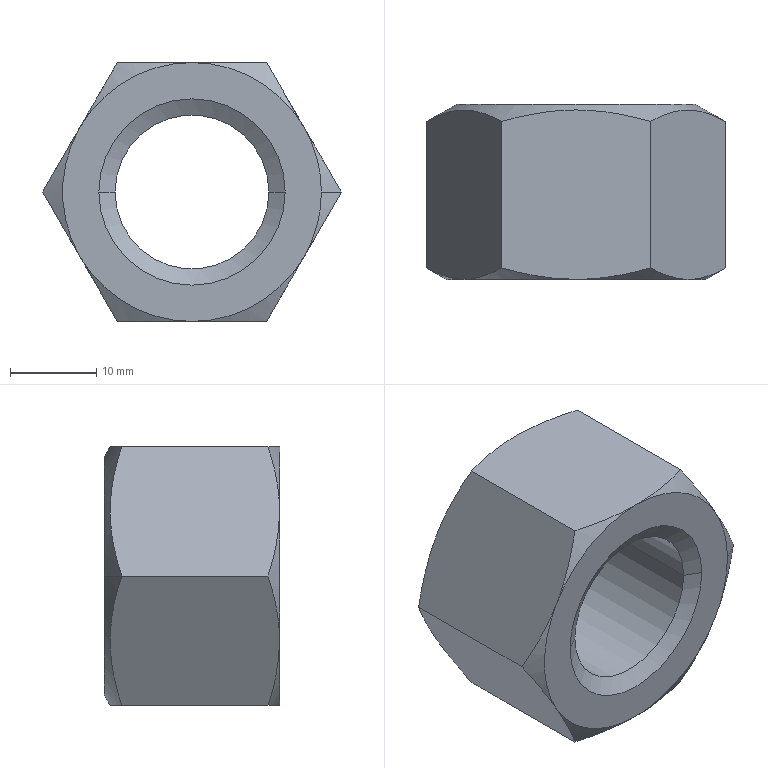Part | NX | features BREP 1 | 1 solid | 23 faces | box 34.641 x 20.3 x 30 mm | volume 10440 mm3 | cone 13 | plane 8 | cylinder 2 | commonest cylinder face diameters 17.835 x2
STEP:
#1=CARTESIAN_POINT('',(58.633,284.435,-38.1));
#2=VERTEX_POINT('',#1);
#3=CARTESIAN_POINT('',(76.468,284.435,-38.1));
#4=VERTEX_POINT('',#3);
#5=CARTESIAN_POINT('',(67.55,284.435,-38.1));
#6=DIRECTION('',(0.,1.,0.));
#7=DIRECTION('',(1.,0.,0.));
#8=AXIS2_PLACEMENT_3D('',#5,#6,#7);
#9=CIRCLE('',#8,8.918);
#10=EDGE_CURVE('',#2,#4,#9,.T.);
#11=ORIENTED_EDGE('',*,*,#10,.F.);
#12=CARTESIAN_POINT('',(56.75,286.317,-38.1));
#13=VERTEX_POINT('',#12);
#14=CARTESIAN_POINT('',(58.633,284.435,-38.1));
#15=DIRECTION('',(-0.7071,0.7071,0.));
#16=VECTOR('',#15,1000.);
#17=LINE('',#14,#16);
#18=EDGE_CURVE('',#2,#13,#17,.T.);
#19=ORIENTED_EDGE('',*,*,#18,.T.);
#20=CARTESIAN_POINT('',(78.35,286.317,-38.1));
#21=VERTEX_POINT('',#20);
#22=CARTESIAN_POINT('',(67.55,286.317,-38.1));
#23=DIRECTION('',(0.,-1.,0.));
#24=DIRECTION('',(1.,0.,0.));
#25=AXIS2_PLACEMENT_3D('',#22,#23,#24);
#26=CIRCLE('',#25,10.8);
#27=EDGE_CURVE('',#21,#13,#26,.T.);
#28=ORIENTED_EDGE('',*,*,#27,.F.);
#29=CARTESIAN_POINT('',(76.468,284.435,-38.1));
#30=DIRECTION('',(0.7071,0.7071,0.));
#31=VECTOR('',#30,1000.);
#32=LINE('',#29,#31);
#33=EDGE_CURVE('',#4,#21,#32,.T.);
#34=ORIENTED_EDGE('',*,*,#33,.F.);
#35=EDGE_LOOP('',(#11,#19,#28,#34));
#36=FACE_BOUND('',#35,.T.);
#37=CARTESIAN_POINT('',(67.55,284.435,-38.1));
#38=DIRECTION('',(0.,1.,0.));
#39=DIRECTION('',(-1.,0.,0.));
#40=AXIS2_PLACEMENT_3D('',#37,#38,#39);
#41=CONICAL_SURFACE('',#40,8.918,0.7854);
#42=ADVANCED_FACE('',(#36),#41,.F.);
#43=CARTESIAN_POINT('',(53.7,286.317,-38.1));
#44=VERTEX_POINT('',#43);
#45=CARTESIAN_POINT('',(81.4,286.317,-38.1));
#46=VERTEX_POINT('',#45);
#47=CARTESIAN_POINT('',(67.55,286.317,-38.1));
#48=DIRECTION('',(0.,-1.,0.));
#49=DIRECTION('',(-1.,0.,0.));
#50=AXIS2_PLACEMENT_3D('',#47,#48,#49);
#51=CIRCLE('',#50,13.85);
#52=EDGE_CURVE('',#44,#46,#51,.T.);
#53=ORIENTED_EDGE('',*,*,#52,.T.);
#54=CARTESIAN_POINT('',(84.871,284.314,-38.1));
#55=VERTEX_POINT('',#54);
#56=CARTESIAN_POINT('',(84.871,284.314,-38.1));
#57=DIRECTION('',(0.866,-0.5,0.));
#58=VECTOR('',#57,1000.);
#59=LINE('',#56,#58);
#60=EDGE_CURVE('',#55,#46,#59,.F.);
#61=ORIENTED_EDGE('',*,*,#60,.F.);
#62=CARTESIAN_POINT('',(76.21,284.314,-53.1));
#63=VERTEX_POINT('',#62);
#64=CARTESIAN_POINT('',(76.21,284.314,-53.1));
#65=CARTESIAN_POINT('',(77.624,285.13,-50.651));
#66=CARTESIAN_POINT('',(80.525,286.176,-45.627));
#67=CARTESIAN_POINT('',(83.455,285.131,-40.552));
#68=CARTESIAN_POINT('',(84.871,284.314,-38.1));
#69=B_SPLINE_CURVE_WITH_KNOTS('',3,(#64,#65,#66,#67,#68),.UNSPECIFIED.,.F.,.F.,(4,1,4),(0.,0.008746,0.01749),.UNSPECIFIED.);
#70=EDGE_CURVE('',#63,#55,#69,.T.);
#71=ORIENTED_EDGE('',*,*,#70,.F.);
#72=CARTESIAN_POINT('',(58.89,284.314,-53.1));
#73=VERTEX_POINT('',#72);
#74=CARTESIAN_POINT('',(58.89,284.314,-53.1));
#75=CARTESIAN_POINT('',(61.718,285.13,-53.1));
#76=CARTESIAN_POINT('',(67.519,286.176,-53.1));
#77=CARTESIAN_POINT('',(73.379,285.131,-53.1));
#78=CARTESIAN_POINT('',(76.21,284.314,-53.1));
#79=B_SPLINE_CURVE_WITH_KNOTS('',3,(#74,#75,#76,#77,#78),.UNSPECIFIED.,.F.,.F.,(4,1,4),(0.,0.008746,0.01749),.UNSPECIFIED.);
#80=EDGE_CURVE('',#73,#63,#79,.T.);
#81=ORIENTED_EDGE('',*,*,#80,.F.);
#82=CARTESIAN_POINT('',(50.229,284.314,-38.1));
#83=VERTEX_POINT('',#82);
#84=CARTESIAN_POINT('',(50.229,284.314,-38.1));
#85=CARTESIAN_POINT('',(51.644,285.13,-40.549));
#86=CARTESIAN_POINT('',(54.544,286.176,-45.573));
#87=CARTESIAN_POINT('',(57.474,285.131,-50.648));
#88=CARTESIAN_POINT('',(58.89,284.314,-53.1));
#89=B_SPLINE_CURVE_WITH_KNOTS('',3,(#84,#85,#86,#87,#88),.UNSPECIFIED.,.F.,.F.,(4,1,4),(0.,0.008746,0.01749),.UNSPECIFIED.);
#90=EDGE_CURVE('',#83,#73,#89,.T.);
#91=ORIENTED_EDGE('',*,*,#90,.F.);
#92=CARTESIAN_POINT('',(50.229,284.314,-38.1));
#93=DIRECTION('',(-0.866,-0.5,0.));
#94=VECTOR('',#93,1000.);
#95=LINE('',#92,#94);
#96=EDGE_CURVE('',#83,#44,#95,.F.);
#97=ORIENTED_EDGE('',*,*,#96,.T.);
#98=EDGE_LOOP('',(#53,#61,#71,#81,#91,#97));
#99=FACE_BOUND('',#98,.T.);
#100=CARTESIAN_POINT('',(67.55,284.314,-38.1));
#101=DIRECTION('',(0.,-1.,0.));
#102=DIRECTION('',(1.,0.,0.));
#103=AXIS2_PLACEMENT_3D('',#100,#101,#102);
#104=CONICAL_SURFACE('',#103,17.321,1.047);
#105=ADVANCED_FACE('',(#99),#104,.T.);
#106=CARTESIAN_POINT('',(58.633,267.104,-38.1));
#107=VERTEX_POINT('',#106);
#108=CARTESIAN_POINT('',(76.468,267.104,-38.1));
#109=VERTEX_POINT('',#108);
#110=CARTESIAN_POINT('',(67.55,267.104,-38.1));
#111=DIRECTION('',(0.,1.,0.));
#112=DIRECTION('',(1.,0.,0.));
#113=AXIS2_PLACEMENT_3D('',#110,#111,#112);
#114=CIRCLE('',#113,8.918);
#115=EDGE_CURVE('',#107,#109,#114,.T.);
#116=ORIENTED_EDGE('',*,*,#115,.T.);
#117=CARTESIAN_POINT('',(78.35,266.017,-38.1));
#118=VERTEX_POINT('',#117);
#119=CARTESIAN_POINT('',(76.468,267.104,-38.1));
#120=DIRECTION('',(0.866,-0.5,0.));
#121=VECTOR('',#120,1000.);
#122=LINE('',#119,#121);
#123=EDGE_CURVE('',#118,#109,#122,.F.);
#124=ORIENTED_EDGE('',*,*,#123,.F.);
#125=CARTESIAN_POINT('',(56.75,266.017,-38.1));
#126=VERTEX_POINT('',#125);
#127=CARTESIAN_POINT('',(67.55,266.017,-38.1));
#128=DIRECTION('',(0.,1.,0.));
#129=DIRECTION('',(1.,0.,0.));
#130=AXIS2_PLACEMENT_3D('',#127,#128,#129);
#131=CIRCLE('',#130,10.8);
#132=EDGE_CURVE('',#126,#118,#131,.T.);
#133=ORIENTED_EDGE('',*,*,#132,.F.);
#134=CARTESIAN_POINT('',(58.633,267.104,-38.1));
#135=DIRECTION('',(-0.866,-0.5,0.));
#136=VECTOR('',#135,1000.);
#137=LINE('',#134,#136);
#138=EDGE_CURVE('',#126,#107,#137,.F.);
#139=ORIENTED_EDGE('',*,*,#138,.T.);
#140=EDGE_LOOP('',(#116,#124,#133,#139));
#141=FACE_BOUND('',#140,.T.);
#142=CARTESIAN_POINT('',(67.55,267.104,-38.1));
#143=DIRECTION('',(0.,-1.,0.));
#144=DIRECTION('',(1.,0.,0.));
#145=AXIS2_PLACEMENT_3D('',#142,#143,#144);
#146=CONICAL_SURFACE('',#145,8.918,1.047);
#147=ADVANCED_FACE('',(#141),#146,.F.);
#148=CARTESIAN_POINT('',(80.54,266.017,-30.6));
#149=VERTEX_POINT('',#148);
#150=CARTESIAN_POINT('',(82.55,266.017,-38.1));
#151=VERTEX_POINT('',#150);
#152=CARTESIAN_POINT('',(67.55,266.017,-38.1));
#153=DIRECTION('',(0.,1.,0.));
#154=DIRECTION('',(1.,0.,0.));
#155=AXIS2_PLACEMENT_3D('',#152,#153,#154);
#156=CIRCLE('',#155,15.);
#157=EDGE_CURVE('',#149,#151,#156,.T.);
#158=ORIENTED_EDGE('',*,*,#157,.T.);
#159=CARTESIAN_POINT('',(84.871,267.357,-38.1));
#160=VERTEX_POINT('',#159);
#161=CARTESIAN_POINT('',(84.871,267.357,-38.1));
#162=DIRECTION('',(0.866,0.5,0.));
#163=VECTOR('',#162,1000.);
#164=LINE('',#161,#163);
#165=EDGE_CURVE('',#151,#160,#164,.T.);
#166=ORIENTED_EDGE('',*,*,#165,.T.);
#167=CARTESIAN_POINT('',(80.54,266.017,-30.6));
#168=CARTESIAN_POINT('',(82.018,266.017,-33.16));
#169=CARTESIAN_POINT('',(83.456,266.54,-35.65));
#170=CARTESIAN_POINT('',(84.871,267.357,-38.1));
#171=B_SPLINE_CURVE_WITH_KNOTS('',3,(#167,#168,#169,#170),.UNSPECIFIED.,.F.,.F.,(4,4),(0.,0.008763),.UNSPECIFIED.);
#172=EDGE_CURVE('',#149,#160,#171,.T.);
#173=ORIENTED_EDGE('',*,*,#172,.F.);
#174=EDGE_LOOP('',(#158,#166,#173));
#175=FACE_BOUND('',#174,.T.);
#176=CARTESIAN_POINT('',(67.55,267.357,-38.1));
#177=DIRECTION('',(0.,1.,0.));
#178=DIRECTION('',(-1.,0.,0.));
#179=AXIS2_PLACEMENT_3D('',#176,#177,#178);
#180=CONICAL_SURFACE('',#179,17.321,1.047);
#181=ADVANCED_FACE('',(#175),#180,.T.);
#182=ORIENTED_EDGE('',*,*,#115,.F.);
#183=CARTESIAN_POINT('',(58.633,266.017,-38.1));
#184=DIRECTION('',(0.,1.,0.));
#185=VECTOR('',#184,1000.);
#186=LINE('',#183,#185);
#187=EDGE_CURVE('',#107,#2,#186,.T.);
#188=ORIENTED_EDGE('',*,*,#187,.T.);
#189=ORIENTED_EDGE('',*,*,#10,.T.);
#190=CARTESIAN_POINT('',(76.468,266.017,-38.1));
#191=DIRECTION('',(0.,1.,0.));
#192=VECTOR('',#191,1000.);
#193=LINE('',#190,#192);
#194=EDGE_CURVE('',#109,#4,#193,.T.);
#195=ORIENTED_EDGE('',*,*,#194,.F.);
#196=EDGE_LOOP('',(#182,#188,#189,#195));
#197=FACE_BOUND('',#196,.T.);
#198=CARTESIAN_POINT('',(67.55,266.017,-38.1));
#199=DIRECTION('',(0.,1.,0.));
#200=DIRECTION('',(-1.,0.,0.));
#201=AXIS2_PLACEMENT_3D('',#198,#199,#200);
#202=CYLINDRICAL_SURFACE('',#201,8.918);
#203=ADVANCED_FACE('',(#197),#202,.F.);
#204=CARTESIAN_POINT('',(76.21,267.357,-23.1));
#205=VERTEX_POINT('',#204);
#206=CARTESIAN_POINT('',(76.21,284.314,-23.1));
#207=VERTEX_POINT('',#206);
#208=CARTESIAN_POINT('',(76.21,266.017,-23.1));
#209=DIRECTION('',(0.,1.,0.));
#210=VECTOR('',#209,1000.);
#211=LINE('',#208,#210);
#212=EDGE_CURVE('',#205,#207,#211,.T.);
#213=ORIENTED_EDGE('',*,*,#212,.T.);
#214=CARTESIAN_POINT('',(58.89,284.314,-23.1));
#215=VERTEX_POINT('',#214);
#216=CARTESIAN_POINT('',(76.21,284.314,-23.1));
#217=CARTESIAN_POINT('',(73.382,285.13,-23.1));
#218=CARTESIAN_POINT('',(67.581,286.176,-23.1));
#219=CARTESIAN_POINT('',(61.721,285.131,-23.1));
#220=CARTESIAN_POINT('',(58.89,284.314,-23.1));
#221=B_SPLINE_CURVE_WITH_KNOTS('',3,(#216,#217,#218,#219,#220),.UNSPECIFIED.,.F.,.F.,(4,1,4),(0.,0.008746,0.01749),.UNSPECIFIED.);
#222=EDGE_CURVE('',#207,#215,#221,.T.);
#223=ORIENTED_EDGE('',*,*,#222,.T.);
#224=CARTESIAN_POINT('',(58.89,267.357,-23.1));
#225=VERTEX_POINT('',#224);
#226=CARTESIAN_POINT('',(58.89,266.017,-23.1));
#227=DIRECTION('',(0.,1.,0.));
#228=VECTOR('',#227,1000.);
#229=LINE('',#226,#228);
#230=EDGE_CURVE('',#225,#215,#229,.T.);
#231=ORIENTED_EDGE('',*,*,#230,.F.);
#232=CARTESIAN_POINT('',(67.55,266.017,-23.1));
#233=VERTEX_POINT('',#232);
#234=CARTESIAN_POINT('',(58.89,267.357,-23.1));
#235=CARTESIAN_POINT('',(61.719,266.54,-23.1));
#236=CARTESIAN_POINT('',(64.594,266.017,-23.1));
#237=CARTESIAN_POINT('',(67.55,266.017,-23.1));
#238=B_SPLINE_CURVE_WITH_KNOTS('',3,(#234,#235,#236,#237),.UNSPECIFIED.,.F.,.F.,(4,4),(0.,0.008763),.UNSPECIFIED.);
#239=EDGE_CURVE('',#225,#233,#238,.T.);
#240=ORIENTED_EDGE('',*,*,#239,.T.);
#241=CARTESIAN_POINT('',(67.55,266.017,-23.1));
#242=CARTESIAN_POINT('',(70.506,266.017,-23.1));
#243=CARTESIAN_POINT('',(73.381,266.54,-23.1));
#244=CARTESIAN_POINT('',(76.21,267.357,-23.1));
#245=B_SPLINE_CURVE_WITH_KNOTS('',3,(#241,#242,#243,#244),.UNSPECIFIED.,.F.,.F.,(4,4),(0.,0.008763),.UNSPECIFIED.);
#246=EDGE_CURVE('',#233,#205,#245,.T.);
#247=ORIENTED_EDGE('',*,*,#246,.T.);
#248=EDGE_LOOP('',(#213,#223,#231,#240,#247));
#249=FACE_BOUND('',#248,.T.);
#250=CARTESIAN_POINT('',(58.89,266.017,-23.1));
#251=DIRECTION('',(0.,0.,1.));
#252=DIRECTION('',(-1.,0.,0.));
#253=AXIS2_PLACEMENT_3D('',#250,#251,#252);
#254=PLANE('',#253);
#255=ADVANCED_FACE('',(#249),#254,.T.);
#256=ORIENTED_EDGE('',*,*,#230,.T.);
#257=CARTESIAN_POINT('',(58.89,284.314,-23.1));
#258=CARTESIAN_POINT('',(57.476,285.13,-25.549));
#259=CARTESIAN_POINT('',(54.575,286.176,-30.573));
#260=CARTESIAN_POINT('',(51.645,285.131,-35.648));
#261=CARTESIAN_POINT('',(50.229,284.314,-38.1));
#262=B_SPLINE_CURVE_WITH_KNOTS('',3,(#257,#258,#259,#260,#261),.UNSPECIFIED.,.F.,.F.,(4,1,4),(0.,0.008746,0.01749),.UNSPECIFIED.);
#263=EDGE_CURVE('',#215,#83,#262,.T.);
#264=ORIENTED_EDGE('',*,*,#263,.T.);
#265=CARTESIAN_POINT('',(50.229,267.357,-38.1));
#266=VERTEX_POINT('',#265);
#267=CARTESIAN_POINT('',(50.229,266.017,-38.1));
#268=DIRECTION('',(0.,1.,0.));
#269=VECTOR('',#268,1000.);
#270=LINE('',#267,#269);
#271=EDGE_CURVE('',#266,#83,#270,.T.);
#272=ORIENTED_EDGE('',*,*,#271,.F.);
#273=CARTESIAN_POINT('',(54.56,266.017,-30.6));
#274=VERTEX_POINT('',#273);
#275=CARTESIAN_POINT('',(50.229,267.357,-38.1));
#276=CARTESIAN_POINT('',(51.644,266.54,-35.65));
#277=CARTESIAN_POINT('',(53.082,266.017,-33.16));
#278=CARTESIAN_POINT('',(54.56,266.017,-30.6));
#279=B_SPLINE_CURVE_WITH_KNOTS('',3,(#275,#276,#277,#278),.UNSPECIFIED.,.F.,.F.,(4,4),(0.,0.008763),.UNSPECIFIED.);
#280=EDGE_CURVE('',#266,#274,#279,.T.);
#281=ORIENTED_EDGE('',*,*,#280,.T.);
#282=CARTESIAN_POINT('',(54.56,266.017,-30.6));
#283=CARTESIAN_POINT('',(56.038,266.017,-28.04));
#284=CARTESIAN_POINT('',(57.475,266.54,-25.55));
#285=CARTESIAN_POINT('',(58.89,267.357,-23.1));
#286=B_SPLINE_CURVE_WITH_KNOTS('',3,(#282,#283,#284,#285),.UNSPECIFIED.,.F.,.F.,(4,4),(0.,0.008763),.UNSPECIFIED.);
#287=EDGE_CURVE('',#274,#225,#286,.T.);
#288=ORIENTED_EDGE('',*,*,#287,.T.);
#289=EDGE_LOOP('',(#256,#264,#272,#281,#288));
#290=FACE_BOUND('',#289,.T.);
#291=CARTESIAN_POINT('',(50.229,266.017,-38.1));
#292=DIRECTION('',(-0.866,0.,0.5));
#293=DIRECTION('',(-0.5,0.,-0.866));
#294=AXIS2_PLACEMENT_3D('',#291,#292,#293);
#295=PLANE('',#294);
#296=ADVANCED_FACE('',(#290),#295,.T.);
#297=ORIENTED_EDGE('',*,*,#271,.T.);
#298=ORIENTED_EDGE('',*,*,#90,.T.);
#299=CARTESIAN_POINT('',(58.89,267.357,-53.1));
#300=VERTEX_POINT('',#299);
#301=CARTESIAN_POINT('',(58.89,266.017,-53.1));
#302=DIRECTION('',(0.,1.,0.));
#303=VECTOR('',#302,1000.);
#304=LINE('',#301,#303);
#305=EDGE_CURVE('',#300,#73,#304,.T.);
#306=ORIENTED_EDGE('',*,*,#305,.F.);
#307=CARTESIAN_POINT('',(54.56,266.017,-45.6));
#308=VERTEX_POINT('',#307);
#309=CARTESIAN_POINT('',(58.89,267.357,-53.1));
#310=CARTESIAN_POINT('',(57.475,266.54,-50.65));
#311=CARTESIAN_POINT('',(56.038,266.017,-48.16));
#312=CARTESIAN_POINT('',(54.56,266.017,-45.6));
#313=B_SPLINE_CURVE_WITH_KNOTS('',3,(#309,#310,#311,#312),.UNSPECIFIED.,.F.,.F.,(4,4),(0.,0.008763),.UNSPECIFIED.);
#314=EDGE_CURVE('',#300,#308,#313,.T.);
#315=ORIENTED_EDGE('',*,*,#314,.T.);
#316=CARTESIAN_POINT('',(54.56,266.017,-45.6));
#317=CARTESIAN_POINT('',(53.082,266.017,-43.04));
#318=CARTESIAN_POINT('',(51.644,266.54,-40.55));
#319=CARTESIAN_POINT('',(50.229,267.357,-38.1));
#320=B_SPLINE_CURVE_WITH_KNOTS('',3,(#316,#317,#318,#319),.UNSPECIFIED.,.F.,.F.,(4,4),(0.,0.008763),.UNSPECIFIED.);
#321=EDGE_CURVE('',#308,#266,#320,.T.);
#322=ORIENTED_EDGE('',*,*,#321,.T.);
#323=EDGE_LOOP('',(#297,#298,#306,#315,#322));
#324=FACE_BOUND('',#323,.T.);
#325=CARTESIAN_POINT('',(58.89,266.017,-53.1));
#326=DIRECTION('',(-0.866,0.,-0.5));
#327=DIRECTION('',(0.5,0.,-0.866));
#328=AXIS2_PLACEMENT_3D('',#325,#326,#327);
#329=PLANE('',#328);
#330=ADVANCED_FACE('',(#324),#329,.T.);
#331=ORIENTED_EDGE('',*,*,#305,.T.);
#332=ORIENTED_EDGE('',*,*,#80,.T.);
#333=CARTESIAN_POINT('',(76.21,267.357,-53.1));
#334=VERTEX_POINT('',#333);
#335=CARTESIAN_POINT('',(76.21,266.017,-53.1));
#336=DIRECTION('',(0.,1.,0.));
#337=VECTOR('',#336,1000.);
#338=LINE('',#335,#337);
#339=EDGE_CURVE('',#334,#63,#338,.T.);
#340=ORIENTED_EDGE('',*,*,#339,.F.);
#341=CARTESIAN_POINT('',(67.55,266.017,-53.1));
#342=VERTEX_POINT('',#341);
#343=CARTESIAN_POINT('',(76.21,267.357,-53.1));
#344=CARTESIAN_POINT('',(73.381,266.54,-53.1));
#345=CARTESIAN_POINT('',(70.506,266.017,-53.1));
#346=CARTESIAN_POINT('',(67.55,266.017,-53.1));
#347=B_SPLINE_CURVE_WITH_KNOTS('',3,(#343,#344,#345,#346),.UNSPECIFIED.,.F.,.F.,(4,4),(0.,0.008763),.UNSPECIFIED.);
#348=EDGE_CURVE('',#334,#342,#347,.T.);
#349=ORIENTED_EDGE('',*,*,#348,.T.);
#350=CARTESIAN_POINT('',(67.55,266.017,-53.1));
#351=CARTESIAN_POINT('',(64.594,266.017,-53.1));
#352=CARTESIAN_POINT('',(61.719,266.54,-53.1));
#353=CARTESIAN_POINT('',(58.89,267.357,-53.1));
#354=B_SPLINE_CURVE_WITH_KNOTS('',3,(#350,#351,#352,#353),.UNSPECIFIED.,.F.,.F.,(4,4),(0.,0.008763),.UNSPECIFIED.);
#355=EDGE_CURVE('',#342,#300,#354,.T.);
#356=ORIENTED_EDGE('',*,*,#355,.T.);
#357=EDGE_LOOP('',(#331,#332,#340,#349,#356));
#358=FACE_BOUND('',#357,.T.);
#359=CARTESIAN_POINT('',(76.21,266.017,-53.1));
#360=DIRECTION('',(0.,0.,-1.));
#361=DIRECTION('',(1.,0.,0.));
#362=AXIS2_PLACEMENT_3D('',#359,#360,#361);
#363=PLANE('',#362);
#364=ADVANCED_FACE('',(#358),#363,.T.);
#365=ORIENTED_EDGE('',*,*,#339,.T.);
#366=ORIENTED_EDGE('',*,*,#70,.T.);
#367=CARTESIAN_POINT('',(84.871,266.017,-38.1));
#368=DIRECTION('',(0.,1.,0.));
#369=VECTOR('',#368,1000.);
#370=LINE('',#367,#369);
#371=EDGE_CURVE('',#160,#55,#370,.T.);
#372=ORIENTED_EDGE('',*,*,#371,.F.);
#373=CARTESIAN_POINT('',(80.54,266.017,-45.6));
#374=VERTEX_POINT('',#373);
#375=CARTESIAN_POINT('',(84.871,267.357,-38.1));
#376=CARTESIAN_POINT('',(83.456,266.54,-40.55));
#377=CARTESIAN_POINT('',(82.018,266.017,-43.04));
#378=CARTESIAN_POINT('',(80.54,266.017,-45.6));
#379=B_SPLINE_CURVE_WITH_KNOTS('',3,(#375,#376,#377,#378),.UNSPECIFIED.,.F.,.F.,(4,4),(0.,0.008763),.UNSPECIFIED.);
#380=EDGE_CURVE('',#160,#374,#379,.T.);
#381=ORIENTED_EDGE('',*,*,#380,.T.);
#382=CARTESIAN_POINT('',(80.54,266.017,-45.6));
#383=CARTESIAN_POINT('',(79.062,266.017,-48.16));
#384=CARTESIAN_POINT('',(77.625,266.54,-50.65));
#385=CARTESIAN_POINT('',(76.21,267.357,-53.1));
#386=B_SPLINE_CURVE_WITH_KNOTS('',3,(#382,#383,#384,#385),.UNSPECIFIED.,.F.,.F.,(4,4),(0.,0.008763),.UNSPECIFIED.);
#387=EDGE_CURVE('',#374,#334,#386,.T.);
#388=ORIENTED_EDGE('',*,*,#387,.T.);
#389=EDGE_LOOP('',(#365,#366,#372,#381,#388));
#390=FACE_BOUND('',#389,.T.);
#391=CARTESIAN_POINT('',(84.871,266.017,-38.1));
#392=DIRECTION('',(0.866,0.,-0.5));
#393=DIRECTION('',(0.5,0.,0.866));
#394=AXIS2_PLACEMENT_3D('',#391,#392,#393);
#395=PLANE('',#394);
#396=ADVANCED_FACE('',(#390),#395,.T.);
#397=ORIENTED_EDGE('',*,*,#371,.T.);
#398=CARTESIAN_POINT('',(84.871,284.314,-38.1));
#399=CARTESIAN_POINT('',(83.456,285.13,-35.651));
#400=CARTESIAN_POINT('',(80.556,286.176,-30.627));
#401=CARTESIAN_POINT('',(77.626,285.131,-25.552));
#402=CARTESIAN_POINT('',(76.21,284.314,-23.1));
#403=B_SPLINE_CURVE_WITH_KNOTS('',3,(#398,#399,#400,#401,#402),.UNSPECIFIED.,.F.,.F.,(4,1,4),(0.,0.008746,0.01749),.UNSPECIFIED.);
#404=EDGE_CURVE('',#55,#207,#403,.T.);
#405=ORIENTED_EDGE('',*,*,#404,.T.);
#406=ORIENTED_EDGE('',*,*,#212,.F.);
#407=CARTESIAN_POINT('',(76.21,267.357,-23.1));
#408=CARTESIAN_POINT('',(77.625,266.54,-25.55));
#409=CARTESIAN_POINT('',(79.062,266.017,-28.04));
#410=CARTESIAN_POINT('',(80.54,266.017,-30.6));
#411=B_SPLINE_CURVE_WITH_KNOTS('',3,(#407,#408,#409,#410),.UNSPECIFIED.,.F.,.F.,(4,4),(0.,0.008763),.UNSPECIFIED.);
#412=EDGE_CURVE('',#205,#149,#411,.T.);
#413=ORIENTED_EDGE('',*,*,#412,.T.);
#414=ORIENTED_EDGE('',*,*,#172,.T.);
#415=EDGE_LOOP('',(#397,#405,#406,#413,#414));
#416=FACE_BOUND('',#415,.T.);
#417=CARTESIAN_POINT('',(76.21,266.017,-23.1));
#418=DIRECTION('',(0.866,0.,0.5));
#419=DIRECTION('',(-0.5,0.,0.866));
#420=AXIS2_PLACEMENT_3D('',#417,#418,#419);
#421=PLANE('',#420);
#422=ADVANCED_FACE('',(#416),#421,.T.);
#423=ORIENTED_EDGE('',*,*,#27,.T.);
#424=CARTESIAN_POINT('',(67.55,286.317,-38.1));
#425=DIRECTION('',(0.,-1.,0.));
#426=DIRECTION('',(1.,0.,0.));
#427=AXIS2_PLACEMENT_3D('',#424,#425,#426);
#428=CIRCLE('',#427,10.8);
#429=EDGE_CURVE('',#13,#21,#428,.T.);
#430=ORIENTED_EDGE('',*,*,#429,.T.);
#431=EDGE_LOOP('',(#423,#430));
#432=FACE_BOUND('',#431,.T.);
#433=ORIENTED_EDGE('',*,*,#52,.F.);
#434=CARTESIAN_POINT('',(67.55,286.317,-38.1));
#435=DIRECTION('',(0.,-1.,0.));
#436=DIRECTION('',(-1.,0.,0.));
#437=AXIS2_PLACEMENT_3D('',#434,#435,#436);
#438=CIRCLE('',#437,13.85);
#439=EDGE_CURVE('',#46,#44,#438,.T.);
#440=ORIENTED_EDGE('',*,*,#439,.F.);
#441=EDGE_LOOP('',(#433,#440));
#442=FACE_BOUND('',#441,.T.);
#443=CARTESIAN_POINT('',(76.21,286.317,-23.1));
#444=DIRECTION('',(0.,1.,0.));
#445=DIRECTION('',(-1.,0.,0.));
#446=AXIS2_PLACEMENT_3D('',#443,#444,#445);
#447=PLANE('',#446);
#448=ADVANCED_FACE('',(#432,#442),#447,.T.);
#449=ORIENTED_EDGE('',*,*,#132,.T.);
#450=CARTESIAN_POINT('',(67.55,266.017,-38.1));
#451=DIRECTION('',(0.,1.,0.));
#452=DIRECTION('',(1.,0.,0.));
#453=AXIS2_PLACEMENT_3D('',#450,#451,#452);
#454=CIRCLE('',#453,10.8);
#455=EDGE_CURVE('',#118,#126,#454,.T.);
#456=ORIENTED_EDGE('',*,*,#455,.T.);
#457=EDGE_LOOP('',(#449,#456));
#458=FACE_BOUND('',#457,.T.);
#459=CARTESIAN_POINT('',(67.55,266.017,-38.1));
#460=DIRECTION('',(0.,1.,0.));
#461=DIRECTION('',(1.,0.,0.));
#462=AXIS2_PLACEMENT_3D('',#459,#460,#461);
#463=CIRCLE('',#462,15.);
#464=EDGE_CURVE('',#374,#342,#463,.T.);
#465=ORIENTED_EDGE('',*,*,#464,.F.);
#466=CARTESIAN_POINT('',(67.55,266.017,-38.1));
#467=DIRECTION('',(0.,1.,0.));
#468=DIRECTION('',(1.,0.,0.));
#469=AXIS2_PLACEMENT_3D('',#466,#467,#468);
#470=CIRCLE('',#469,15.);
#471=EDGE_CURVE('',#151,#374,#470,.T.);
#472=ORIENTED_EDGE('',*,*,#471,.F.);
#473=ORIENTED_EDGE('',*,*,#157,.F.);
#474=CARTESIAN_POINT('',(67.55,266.017,-38.1));
#475=DIRECTION('',(0.,1.,0.));
#476=DIRECTION('',(1.,0.,0.));
#477=AXIS2_PLACEMENT_3D('',#474,#475,#476);
#478=CIRCLE('',#477,15.);
#479=EDGE_CURVE('',#233,#149,#478,.T.);
#480=ORIENTED_EDGE('',*,*,#479,.F.);
#481=CARTESIAN_POINT('',(67.55,266.017,-38.1));
#482=DIRECTION('',(0.,1.,0.));
#483=DIRECTION('',(1.,0.,0.));
#484=AXIS2_PLACEMENT_3D('',#481,#482,#483);
#485=CIRCLE('',#484,15.);
#486=EDGE_CURVE('',#274,#233,#485,.T.);
#487=ORIENTED_EDGE('',*,*,#486,.F.);
#488=CARTESIAN_POINT('',(67.55,266.017,-38.1));
#489=DIRECTION('',(0.,1.,0.));
#490=DIRECTION('',(1.,0.,0.));
#491=AXIS2_PLACEMENT_3D('',#488,#489,#490);
#492=CIRCLE('',#491,15.);
#493=EDGE_CURVE('',#308,#274,#492,.T.);
#494=ORIENTED_EDGE('',*,*,#493,.F.);
#495=CARTESIAN_POINT('',(67.55,266.017,-38.1));
#496=DIRECTION('',(0.,1.,0.));
#497=DIRECTION('',(1.,0.,0.));
#498=AXIS2_PLACEMENT_3D('',#495,#496,#497);
#499=CIRCLE('',#498,15.);
#500=EDGE_CURVE('',#342,#308,#499,.T.);
#501=ORIENTED_EDGE('',*,*,#500,.F.);
#502=EDGE_LOOP('',(#465,#472,#473,#480,#487,#494,#501));
#503=FACE_BOUND('',#502,.T.);
#504=CARTESIAN_POINT('',(76.21,266.017,-23.1));
#505=DIRECTION('',(0.,1.,0.));
#506=DIRECTION('',(-1.,0.,0.));
#507=AXIS2_PLACEMENT_3D('',#504,#505,#506);
#508=PLANE('',#507);
#509=ADVANCED_FACE('',(#458,#503),#508,.F.);
#510=ORIENTED_EDGE('',*,*,#187,.F.);
#511=CARTESIAN_POINT('',(67.55,267.104,-38.1));
#512=DIRECTION('',(0.,1.,0.));
#513=DIRECTION('',(1.,0.,0.));
#514=AXIS2_PLACEMENT_3D('',#511,#512,#513);
#515=CIRCLE('',#514,8.918);
#516=EDGE_CURVE('',#109,#107,#515,.T.);
#517=ORIENTED_EDGE('',*,*,#516,.F.);
#518=ORIENTED_EDGE('',*,*,#194,.T.);
#519=CARTESIAN_POINT('',(67.55,284.435,-38.1));
#520=DIRECTION('',(0.,1.,0.));
#521=DIRECTION('',(1.,0.,0.));
#522=AXIS2_PLACEMENT_3D('',#519,#520,#521);
#523=CIRCLE('',#522,8.918);
#524=EDGE_CURVE('',#4,#2,#523,.T.);
#525=ORIENTED_EDGE('',*,*,#524,.T.);
#526=EDGE_LOOP('',(#510,#517,#518,#525));
#527=FACE_BOUND('',#526,.T.);
#528=CARTESIAN_POINT('',(67.55,266.017,-38.1));
#529=DIRECTION('',(0.,1.,0.));
#530=DIRECTION('',(-1.,0.,0.));
#531=AXIS2_PLACEMENT_3D('',#528,#529,#530);
#532=CYLINDRICAL_SURFACE('',#531,8.918);
#533=ADVANCED_FACE('',(#527),#532,.F.);
#534=ORIENTED_EDGE('',*,*,#165,.F.);
#535=ORIENTED_EDGE('',*,*,#471,.T.);
#536=ORIENTED_EDGE('',*,*,#380,.F.);
#537=EDGE_LOOP('',(#534,#535,#536));
#538=FACE_BOUND('',#537,.T.);
#539=CARTESIAN_POINT('',(67.55,267.357,-38.1));
#540=DIRECTION('',(0.,1.,0.));
#541=DIRECTION('',(-1.,0.,0.));
#542=AXIS2_PLACEMENT_3D('',#539,#540,#541);
#543=CONICAL_SURFACE('',#542,17.321,1.047);
#544=ADVANCED_FACE('',(#538),#543,.T.);
#545=ORIENTED_EDGE('',*,*,#479,.T.);
#546=ORIENTED_EDGE('',*,*,#412,.F.);
#547=ORIENTED_EDGE('',*,*,#246,.F.);
#548=EDGE_LOOP('',(#545,#546,#547));
#549=FACE_BOUND('',#548,.T.);
#550=CARTESIAN_POINT('',(67.55,267.357,-38.1));
#551=DIRECTION('',(0.,1.,0.));
#552=DIRECTION('',(-1.,0.,0.));
#553=AXIS2_PLACEMENT_3D('',#550,#551,#552);
#554=CONICAL_SURFACE('',#553,17.321,1.047);
#555=ADVANCED_FACE('',(#549),#554,.T.);
#556=ORIENTED_EDGE('',*,*,#486,.T.);
#557=ORIENTED_EDGE('',*,*,#239,.F.);
#558=ORIENTED_EDGE('',*,*,#287,.F.);
#559=EDGE_LOOP('',(#556,#557,#558));
#560=FACE_BOUND('',#559,.T.);
#561=CARTESIAN_POINT('',(67.55,267.357,-38.1));
#562=DIRECTION('',(0.,1.,0.));
#563=DIRECTION('',(-1.,0.,0.));
#564=AXIS2_PLACEMENT_3D('',#561,#562,#563);
#565=CONICAL_SURFACE('',#564,17.321,1.047);
#566=ADVANCED_FACE('',(#560),#565,.T.);
#567=ORIENTED_EDGE('',*,*,#493,.T.);
#568=ORIENTED_EDGE('',*,*,#280,.F.);
#569=ORIENTED_EDGE('',*,*,#321,.F.);
#570=EDGE_LOOP('',(#567,#568,#569));
#571=FACE_BOUND('',#570,.T.);
#572=CARTESIAN_POINT('',(67.55,267.357,-38.1));
#573=DIRECTION('',(0.,1.,0.));
#574=DIRECTION('',(-1.,0.,0.));
#575=AXIS2_PLACEMENT_3D('',#572,#573,#574);
#576=CONICAL_SURFACE('',#575,17.321,1.047);
#577=ADVANCED_FACE('',(#571),#576,.T.);
#578=ORIENTED_EDGE('',*,*,#355,.F.);
#579=ORIENTED_EDGE('',*,*,#500,.T.);
#580=ORIENTED_EDGE('',*,*,#314,.F.);
#581=EDGE_LOOP('',(#578,#579,#580));
#582=FACE_BOUND('',#581,.T.);
#583=CARTESIAN_POINT('',(67.55,267.357,-38.1));
#584=DIRECTION('',(0.,1.,0.));
#585=DIRECTION('',(-1.,0.,0.));
#586=AXIS2_PLACEMENT_3D('',#583,#584,#585);
#587=CONICAL_SURFACE('',#586,17.321,1.047);
#588=ADVANCED_FACE('',(#582),#587,.T.);
#589=ORIENTED_EDGE('',*,*,#387,.F.);
#590=ORIENTED_EDGE('',*,*,#464,.T.);
#591=ORIENTED_EDGE('',*,*,#348,.F.);
#592=EDGE_LOOP('',(#589,#590,#591));
#593=FACE_BOUND('',#592,.T.);
#594=CARTESIAN_POINT('',(67.55,267.357,-38.1));
#595=DIRECTION('',(0.,1.,0.));
#596=DIRECTION('',(-1.,0.,0.));
#597=AXIS2_PLACEMENT_3D('',#594,#595,#596);
#598=CONICAL_SURFACE('',#597,17.321,1.047);
#599=ADVANCED_FACE('',(#593),#598,.T.);
#600=ORIENTED_EDGE('',*,*,#123,.T.);
#601=ORIENTED_EDGE('',*,*,#516,.T.);
#602=ORIENTED_EDGE('',*,*,#138,.F.);
#603=ORIENTED_EDGE('',*,*,#455,.F.);
#604=EDGE_LOOP('',(#600,#601,#602,#603));
#605=FACE_BOUND('',#604,.T.);
#606=CARTESIAN_POINT('',(67.55,267.104,-38.1));
#607=DIRECTION('',(0.,-1.,0.));
#608=DIRECTION('',(1.,0.,0.));
#609=AXIS2_PLACEMENT_3D('',#606,#607,#608);
#610=CONICAL_SURFACE('',#609,8.918,1.047);
#611=ADVANCED_FACE('',(#605),#610,.F.);
#612=ORIENTED_EDGE('',*,*,#60,.T.);
#613=ORIENTED_EDGE('',*,*,#439,.T.);
#614=ORIENTED_EDGE('',*,*,#96,.F.);
#615=ORIENTED_EDGE('',*,*,#263,.F.);
#616=ORIENTED_EDGE('',*,*,#222,.F.);
#617=ORIENTED_EDGE('',*,*,#404,.F.);
#618=EDGE_LOOP('',(#612,#613,#614,#615,#616,#617));
#619=FACE_BOUND('',#618,.T.);
#620=CARTESIAN_POINT('',(67.55,284.314,-38.1));
#621=DIRECTION('',(0.,-1.,0.));
#622=DIRECTION('',(1.,0.,0.));
#623=AXIS2_PLACEMENT_3D('',#620,#621,#622);
#624=CONICAL_SURFACE('',#623,17.321,1.047);
#625=ADVANCED_FACE('',(#619),#624,.T.);
#626=ORIENTED_EDGE('',*,*,#18,.F.);
#627=ORIENTED_EDGE('',*,*,#524,.F.);
#628=ORIENTED_EDGE('',*,*,#33,.T.);
#629=ORIENTED_EDGE('',*,*,#429,.F.);
#630=EDGE_LOOP('',(#626,#627,#628,#629));
#631=FACE_BOUND('',#630,.T.);
#632=CARTESIAN_POINT('',(67.55,284.435,-38.1));
#633=DIRECTION('',(0.,1.,0.));
#634=DIRECTION('',(-1.,0.,0.));
#635=AXIS2_PLACEMENT_3D('',#632,#633,#634);
#636=CONICAL_SURFACE('',#635,8.918,0.7854);
#637=ADVANCED_FACE('',(#631),#636,.F.);
#638=CLOSED_SHELL('',(#42,#105,#147,#181,#203,#255,#296,#330,#364,#396,#422,#448,#509,#533,#544,#555,#566,#577,#588,#599,#611,#625,#637));
#639=MANIFOLD_SOLID_BREP('',#638);
#640=(LENGTH_UNIT()NAMED_UNIT(*)SI_UNIT(.MILLI.,.METRE.));
#641=UNCERTAINTY_MEASURE_WITH_UNIT(LENGTH_MEASURE(0.0508),#640,'','');
#642=(NAMED_UNIT(*)PLANE_ANGLE_UNIT()SI_UNIT($,.RADIAN.));
#643=(NAMED_UNIT(*)SI_UNIT($,.STERADIAN.)SOLID_ANGLE_UNIT());
#644=(GEOMETRIC_REPRESENTATION_CONTEXT(3)GLOBAL_UNCERTAINTY_ASSIGNED_CONTEXT((#641))GLOBAL_UNIT_ASSIGNED_CONTEXT((#640,#642,#643))REPRESENTATION_CONTEXT('',''));
#645=ADVANCED_BREP_SHAPE_REPRESENTATION('',(#639),#644);